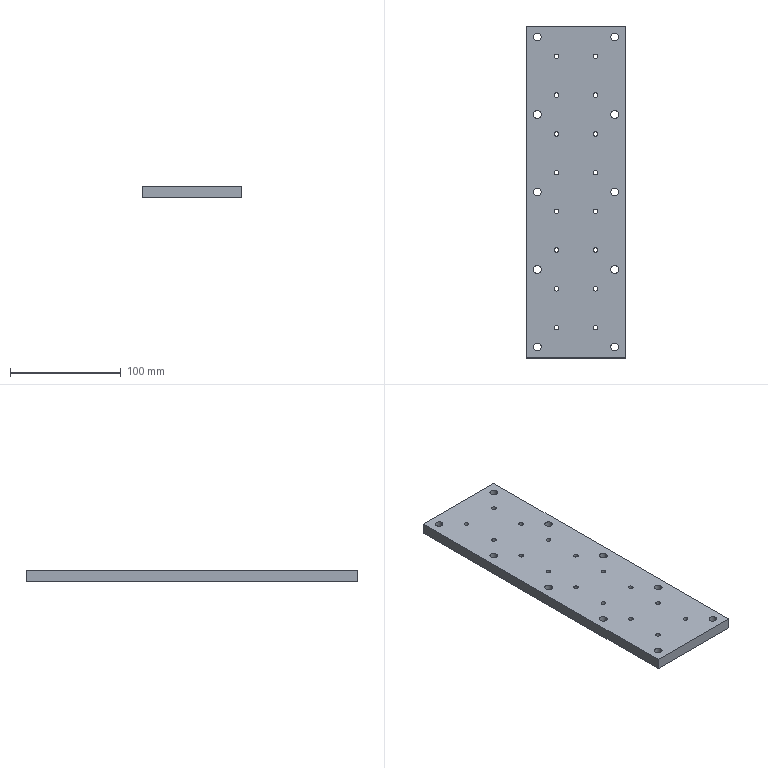Part | SolidWorks | features LPattern 3, HoleWzd 2, Extrusion 1 | 1 solid | 58 faces | box 90 x 300 x 10 mm | volume 263935 mm3 | cylinder 52 | plane 6 | commonest cylinder face diameters 4.2 x32 7 x20